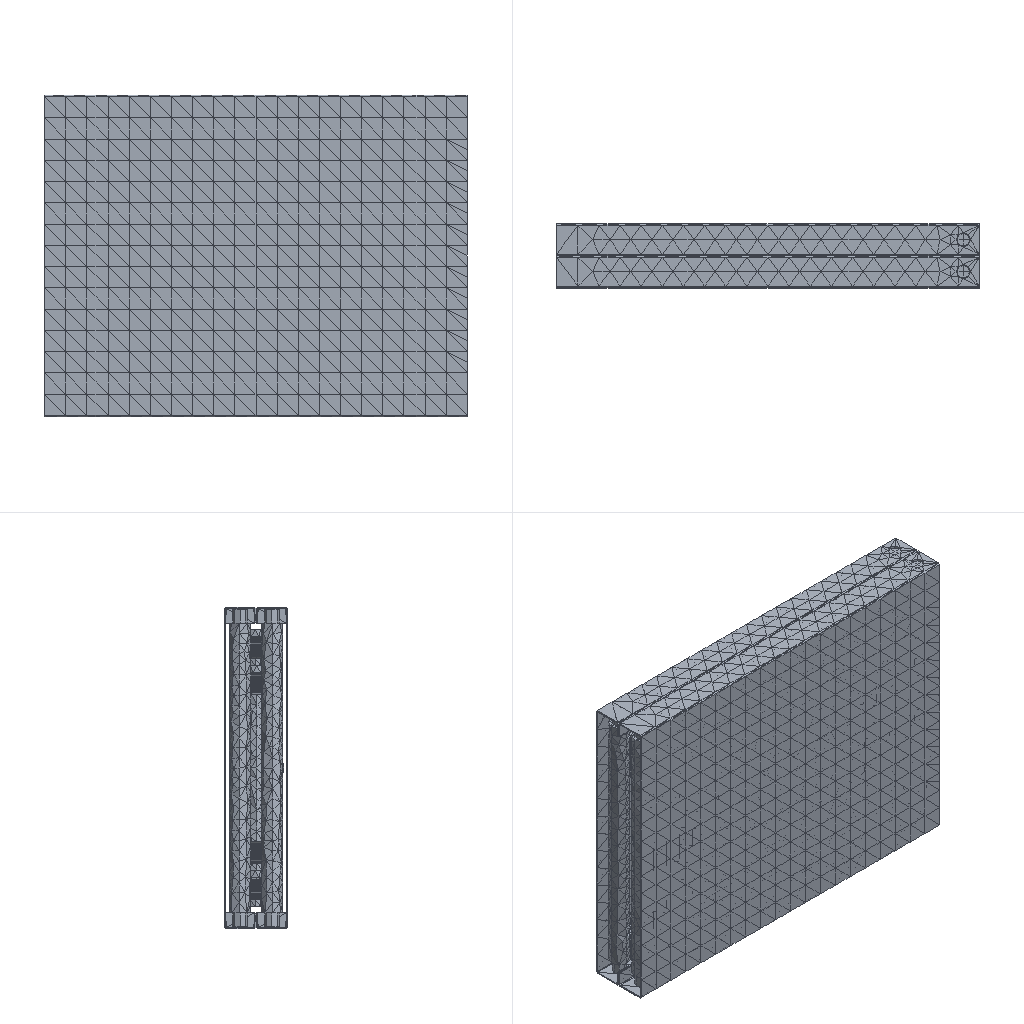Simulation study | abaqus
Set-up summary:
category,name,step,type,value,unit,region
solver,abaqus
solver,version,,,Abaqus/Explicit 2020
units,not stated in the deck,,not stated
analysis,deck,,transient,transient
load_step,Step-1,Step-1,transient
load_step,requested,,,1
mesh,nodes,,,15230
mesh,elements,,,42276
element_type,C3D4,,solid,41198
element_type,C3D8R,,solid,1078
load,load commands in deck,,count,3
bc,support commands in deck,,count,12
material,AI,,in results
check,setup vs results,,match,"per instance, exact: element labels, types and connectivity; labels of the nodes the elements use; coordinates not compared"
Abaqus input file, long lists of numbers shortened:
*Heading
** Job name: Job-1 Model name: Model-1
** Generated by: Abaqus/CAE 2020
*Preprint, echo=NO, model=NO, history=NO, contact=NO
**
** PARTS
**
*Part, name=WORK-1
*Node
      1,   7.262,   37.636,        -192.
      2,  0.8978,          35.,        -192.
** (205 more lines like these left out)
*Element, type=C3D8R
 1,  11,  12,  18,  10,   2,   3,   9,   1
 2,  14,  15,  18,  12,   5,   6,   9,   3
** (86 more lines like these left out)
*Nset, nset=Set-2, generate
   1,  207,    1
*Elset, elset=Set-2, generate
  1,  88,   1
** Section: Section-1
*Solid Section, elset=Set-2, material=AI
,
*End Part
**
*Part, name=WORK-2
*Node
      1,   49.212,   40.328,         -40.
      2,   47.261,   37.408,         -40.
** (872 more lines like these left out)
*Element, type=C3D8R
  1,  69,  42,  43,  56,  31,   4,   5,  18
  2,  43,  44,  70,  56,   5,   6,  32,  18
** (636 more lines like these left out)
*Nset, nset=Set-2, generate
   1,  874,    1
*Elset, elset=Set-2, generate
   1,  638,    1
** Section: Section-1
*Solid Section, elset=Set-2, material=AI
,
*End Part
**
*Part, name=WORK-3
*Node
      1,   221.697,    26.355,         13.5
      2,   221.697,    26.355,        -13.5
** (710 more lines like these left out)
*Element, type=C3D4
   1, 627, 628, 121, 610
   2, 627, 629, 630, 631
** (2272 more lines like these left out)
*Nset, nset=Set-4, generate
   1,  712,    1
*Elset, elset=Set-4, generate
    1,  2274,     1
** Section: Section-1
*Solid Section, elset=Set-4, material=AI
,
*End Part
**
*Part, name=WORK-4
*Node
      1,   220.068,   26.512,        -12.5
      2,   221.266,   38.955,           0.
** (209 more lines like these left out)
*Element, type=C3D4
  1, 191,  70,  71,  78
  2,  45, 192,  38,  37
** (585 more lines like these left out)
*Nset, nset=Set-4, generate
   1,  211,    1
*Elset, elset=Set-4, generate
   1,  587,    1
** Section: Section-1
*Solid Section, elset=Set-4, material=AI
,
*End Part
**
*Part, name=WORK-5
*Node
      1,  -261.84,   59.636,      -220.25
      2,  -268.204,          57.,      -220.25
** (205 more lines like these left out)
*Element, type=C3D8R
 1,  10,  11,  18,  13,   1,   2,   9,   4
 2,  17,  13,  18,  16,   8,   4,   9,   7
** (86 more lines like these left out)
*Nset, nset=Set-2, generate
   1,  207,    1
*Elset, elset=Set-2, generate
  1,  88,   1
** Section: Section-1
*Solid Section, elset=Set-2, material=AI
,
*End Part
**
*Part, name=WORK-6
*Node
      1,   276.364,   59.636,      -220.25
      2,         270.,          57.,      -220.25
** (205 more lines like these left out)
*Element, type=C3D8R
 1,  10,  11,  18,  13,   1,   2,   9,   4
 2,  12,  14,  18,  11,   3,   5,   9,   2
** (86 more lines like these left out)
*Nset, nset=Set-1, generate
   1,  207,    1
*Elset, elset=Set-1, generate
  1,  88,   1
** Section: Section-1
*Solid Section, elset=Set-1, material=AI
,
*End Part
**
*Part, name=WORK-7
*Node
      1,   276.364,   15.636,      -220.25
      2,         270.,          13.,      -220.25
** (205 more lines like these left out)
*Element, type=C3D8R
 1,  18,  11,  12,  14,   9,   2,   3,   5
 2,  10,  11,  18,  13,   1,   2,   9,   4
** (86 more lines like these left out)
*Nset, nset=Set-1, generate
   1,  207,    1
*Elset, elset=Set-1, generate
  1,  88,   1
** Section: Section-1
*Solid Section, elset=Set-1, material=AI
,
*End Part
**
*Part, name=WORK-8
*Node
      1,  -261.84,   15.636,      -220.25
      2,  -268.204,          13.,      -220.25
** (205 more lines like these left out)
*Element, type=C3D8R
 1,  18,  11,  12,  14,   9,   2,   3,   5
 2,  10,  11,  18,  13,   1,   2,   9,   4
** (86 more lines like these left out)
*Nset, nset=Set-1, generate
   1,  207,    1
*Elset, elset=Set-1, generate
  1,  88,   1
** Section: Section-1
*Solid Section, elset=Set-1, material=AI
,
*End Part
**
*Part, name=WORK-11
*Node
      1,         242.,          86.,      -200.25
      2,         242.,          86.,      -219.25
** (1151 more lines like these left out)
*Element, type=C3D4
   1, 1136,   63,   62,  243
   2,    7,   58,   10,   26
** (3214 more lines like these left out)
*Nset, nset=Set-1, generate
    1,  1153,     1
*Elset, elset=Set-1, generate
    1,  3216,     1
** Section: Section-1
*Solid Section, elset=Set-1, material=AI
,
*End Part
**
*Part, name=WORK-12
*Node
      1,  0.08297,   53.967,         142.
      2,  -9.069,   43.185,         142.
** (5124 more lines like these left out)
*Element, type=C3D4
    1, 4402, 1843, 4209, 1844
    2, 1441, 1803, 4209, 1804
** (16189 more lines like these left out)
*Nset, nset=Set-1, generate
    1,  5126,     1
*Elset, elset=Set-1, generate
     1,  16191,      1
** Section: Section-1
*Solid Section, elset=Set-1, material=AI
,
*End Part
**
*Part, name=WORK-15
*Node
      1,  -278.171,   66.815,       200.25
      2,  -258.238,   65.185,       200.25
** (4965 more lines like these left out)
*Element, type=C3D4
    1, 3918, 4688, 4421, 3917
    2, 4689, 3577, 4690, 4348
** (15720 more lines like these left out)
*Nset, nset=Set-1, generate
    1,  4967,     1
*Elset, elset=Set-1, generate
     1,  15722,      1
** Section: Section-1
*Solid Section, elset=Set-1, material=AI
,
*End Part
**
*Part, name=WORK-16
*Node
      1,         242.,           2.,       200.25
      2,         242.,           2.,       219.25
** (1150 more lines like these left out)
*Element, type=C3D4
   1,  388, 1136,   26,  407
   2, 1013,  790,  800,  999
** (3206 more lines like these left out)
*Nset, nset=Set-6, generate
    1,  1152,     1
*Elset, elset=Set-6, generate
    1,  3208,     1
** Section: Section-1
*Solid Section, elset=Set-6, material=AI
,
*End Part
**
**
** ASSEMBLY
**
*Assembly, name=Assembly
**
*Instance, name=WORK-1-1, part=WORK-1
*End Instance
**
*Instance, name=WORK-2-1, part=WORK-2
*End Instance
**
*Instance, name=WORK-3-1, part=WORK-3
*End Instance
**
*Instance, name=WORK-4-1, part=WORK-4
*End Instance
**
*Instance, name=WORK-5-1, part=WORK-5
*End Instance
**
*Instance, name=WORK-6-1, part=WORK-6
*End Instance
**
*Instance, name=WORK-7-1, part=WORK-7
*End Instance
**
*Instance, name=WORK-8-1, part=WORK-8
*End Instance
**
*Instance, name=WORK-11-1, part=WORK-11
*End Instance
**
*Instance, name=WORK-12-1, part=WORK-12
*End Instance
**
*Instance, name=WORK-15-1, part=WORK-15
*End Instance
**
*Instance, name=WORK-16-1, part=WORK-16
*End Instance
**
*Node
      1,           0.,         100.,           0.
*Nset, nset=Set-1, instance=WORK-16-1
   15,   16,   46,   47,   77,   78,   79,   80,   81,   82,   83,   84,   85,   86,   87,   88
   89,   90,  389,  390,  391,  392,  393,  394,  395,  396,  397,  398,  399,  400,  401,  402
** (20 more lines like these left out)
*Elset, elset=Set-1, instance=WORK-16-1
   19,   34,   38,   48,   50,  234,  236,  244,  245,  247,  248,  250,  252,  253,  254,  256
  260,  265,  266,  270,  272,  273,  274,  278,  279,  284,  290,  299,  308,  309,  313,  315
** (37 more lines like these left out)
*Nset, nset=Set-2, instance=WORK-11-1
   15,   16,   46,   47,   77,   78,   79,   80,   81,   82,   83,   84,   85,   86,   87,   88
   89,   90,  389,  390,  391,  392,  393,  394,  395,  396,  397,  398,  399,  400,  401,  402
** (20 more lines like these left out)
*Elset, elset=Set-2, instance=WORK-11-1
    7,    8,   60,   64,   67,   82,   94,  146,  261,  263,  266,  267,  276,  278,  279,  283
  284,  285,  287,  292,  297,  298,  302,  304,  310,  314,  315,  320,  322,  333,  336,  339
** (37 more lines like these left out)
*Nset, nset=Set-4
 1,
*Nset, nset=Set-5, instance=WORK-7-1
   1,   2,   3,   4,   5,   6,   7,   8,   9, 199, 200, 201, 202, 203, 204, 205
 206, 207
*Nset, nset=Set-5, instance=WORK-8-1
   1,   2,   3,   4,   5,   6,   7,   8,   9, 199, 200, 201, 202, 203, 204, 205
 206, 207
*Elset, elset=Set-5, instance=WORK-7-1
  1,  2,  3,  4, 85, 86, 87, 88
*Elset, elset=Set-5, instance=WORK-8-1
  1,  2,  3,  4, 85, 86, 87, 88
*Nset, nset=Set-6
 1,
*Nset, nset=m_Set-3
 1,
*Elset, elset=_m_Surf-1_S2, internal, instance=WORK-5-1, generate
 1,  4,  1
*Surface, type=ELEMENT, name=m_Surf-1
_m_Surf-1_S2, S2
*Elset, elset=_m_Surf-3_S1, internal, instance=WORK-5-1, generate
 85,  88,   1
*Surface, type=ELEMENT, name=m_Surf-3
_m_Surf-3_S1, S1
*Elset, elset=_m_Surf-5_S1, internal, instance=WORK-8-1, generate
 85,  88,   1
*Surface, type=ELEMENT, name=m_Surf-5
_m_Surf-5_S1, S1
*Elset, elset=_m_Surf-7_S2, internal, instance=WORK-8-1, generate
 1,  4,  1
*Surface, type=ELEMENT, name=m_Surf-7
_m_Surf-7_S2, S2
*Elset, elset=_m_Surf-9_S2, internal, instance=WORK-1-1, generate
 1,  4,  1
*Surface, type=ELEMENT, name=m_Surf-9
_m_Surf-9_S2, S2
*Elset, elset=_m_Surf-11_S1, internal, instance=WORK-1-1, generate
 85,  88,   1
*Surface, type=ELEMENT, name=m_Surf-11
_m_Surf-11_S1, S1
*Elset, elset=_m_Surf-13_S1, internal, instance=WORK-2-1, generate
 610,  638,    1
*Surface, type=ELEMENT, name=m_Surf-13
_m_Surf-13_S1, S1
*Elset, elset=_m_Surf-15_S2, internal, instance=WORK-2-1, generate
  1,  29,   1
*Surface, type=ELEMENT, name=m_Surf-15
_m_Surf-15_S2, S2
*Elset, elset=_m_Surf-17_S2, internal, instance=WORK-7-1, generate
 1,  4,  1
*Surface, type=ELEMENT, name=m_Surf-17
_m_Surf-17_S2, S2
*Elset, elset=_m_Surf-19_S1, internal, instance=WORK-7-1, generate
 85,  88,   1
*Surface, type=ELEMENT, name=m_Surf-19
_m_Surf-19_S1, S1
*Elset, elset=_m_Surf-22_S3, internal, instance=WORK-11-1
 1265, 1636, 1824, 1874, 1936, 1947, 1950, 1954, 1958, 1963, 1969, 1971, 1973, 1976, 1979, 1980
 1982, 1983, 1986, 1988, 1991, 1998, 2003, 2005, 2006, 2008, 2025, 2251, 2301, 2337, 2634, 3199
*Elset, elset=_m_Surf-22_S1, internal, instance=WORK-11-1
 1934,
*Elset, elset=_m_Surf-22_S4, internal, instance=WORK-11-1
 1941, 2218, 2557
*Surface, type=ELEMENT, name=m_Surf-22
_m_Surf-22_S3, S3
_m_Surf-22_S1, S1
_m_Surf-22_S4, S4
*Elset, elset=_s_Surf-9_S3, internal, instance=WORK-15-1
   19,   20, 4468, 8664, 8738, 9003
*Elset, elset=_s_Surf-9_S4, internal, instance=WORK-15-1
   917,  8114,  8551,  8679,  8687,  8734,  9651, 12450
*Elset, elset=_s_Surf-9_S2, internal, instance=WORK-15-1
  7329,  8970, 11381, 14219
*Elset, elset=_s_Surf-9_S1, internal, instance=WORK-15-1
 9655,
*Surface, type=ELEMENT, name=s_Surf-9
_s_Surf-9_S3, S3
_s_Surf-9_S4, S4
_s_Surf-9_S2, S2
_s_Surf-9_S1, S1
*Elset, elset=_s_Surf-11_S3, internal, instance=WORK-15-1
   204,  1697,  6734,  7453,  8763,  8825,  8840,  9844,  9986,  9988,  9997,  9998, 10074, 10289
*Elset, elset=_s_Surf-11_S4, internal, instance=WORK-15-1
   654,  1522,  9991, 10290
*Elset, elset=_s_Surf-11_S1, internal, instance=WORK-15-1
 12418,
*Surface, type=ELEMENT, name=s_Surf-11
_s_Surf-11_S3, S3
_s_Surf-11_S4, S4
_s_Surf-11_S1, S1
*Elset, elset=_s_Surf-13_S3, internal, instance=WORK-12-1
    39,   233,   457,  1169,  1170,  9256,  9276,  9284,  9342,  9351,  9464,  9510,  9515,  9607,  9940, 11445
 11625,
*Elset, elset=_s_Surf-13_S2, internal, instance=WORK-12-1
 440,
*Elset, elset=_s_Surf-13_S1, internal, instance=WORK-12-1
  442, 9272
*Elset, elset=_s_Surf-13_S4, internal, instance=WORK-12-1
  1168,  9617,  9901, 11439
*Surface, type=ELEMENT, name=s_Surf-13
_s_Surf-13_S3, S3
_s_Surf-13_S2, S2
_s_Surf-13_S4, S4
_s_Surf-13_S1, S1
*Elset, elset=_s_Surf-15_S4, internal, instance=WORK-12-1
    30,  7769,  7956, 12024, 15156
*Elset, elset=_s_Surf-15_S3, internal, instance=WORK-12-1
    77,   187,  1341,  3155,  5025,  5391,  6906,  6913,  7975, 10011, 12041, 15675, 15787, 15804, 15808, 15815
 15823,
*Elset, elset=_s_Surf-15_S2, internal, instance=WORK-12-1
 5422,
*Elset, elset=_s_Surf-15_S1, internal, instance=WORK-12-1
 15677,
*Surface, type=ELEMENT, name=s_Surf-15
_s_Surf-15_S4, S4
_s_Surf-15_S3, S3
_s_Surf-15_S2, S2
_s_Surf-15_S1, S1
*Elset, elset=_s_Surf-17_S4, internal, instance=WORK-16-1
   36,  121,  125,  128,  145,  146,  147,  148,  150,  167,  170,  171,  173,  179,  187,  208
  209,  217,  221,  224,  846, 1879, 1990, 2024, 2135, 2240, 2241, 2579, 2637, 2670, 2681, 2712
** (1 more lines like these left out)
*Elset, elset=_s_Surf-17_S3, internal, instance=WORK-16-1
   51,   55,   76,  158,  169,  175,  211,  769, 2086, 2108, 2157, 2160, 2552
*Elset, elset=_s_Surf-17_S1, internal, instance=WORK-16-1
   68,  116,  186,  188,  191,  214,  996, 1421, 1827, 2286, 2642, 2690, 2727, 2981, 2986, 2987
 2997, 3037
*Elset, elset=_s_Surf-17_S2, internal, instance=WORK-16-1
   89,  124,  140,  168,  184,  192,  199,  218,  222,  267,  351,  480, 1050, 1137, 2080, 2536
 2555, 2583, 2892, 2896, 2897, 2954, 2959
*Surface, type=ELEMENT, name=s_Surf-17
_s_Surf-17_S4, S4
_s_Surf-17_S3, S3
_s_Surf-17_S2, S2
_s_Surf-17_S1, S1
*Elset, elset=_s_Surf-19_S3, internal, instance=WORK-16-1
   21,   74,   75,  924, 1760, 1906, 1979, 2199
*Elset, elset=_s_Surf-19_S2, internal, instance=WORK-16-1
  511, 1047, 1707, 1711, 1715, 1719, 1723, 1728, 1751, 1828, 1851, 1893, 1897, 1957, 1959, 1971
 1974, 2015, 2151, 2190, 2360, 2384
*Elset, elset=_s_Surf-19_S4, internal, instance=WORK-16-1
  607, 1714, 1741, 1782, 1792, 1794, 1802, 1818, 1835, 1853, 1868, 1875, 1907, 1910, 1922, 1926
 1949, 1953, 1996, 2019, 2025, 2105, 2269, 2296, 2301, 2303, 2308, 2317, 2321, 2325, 3136
*Elset, elset=_s_Surf-19_S1, internal, instance=WORK-16-1
 1708, 1709, 1718, 1722, 1732, 1735, 1742, 1744, 1750, 1769, 1780, 1781, 1785, 1805, 1809, 1813
 1816, 1819, 1837, 1925, 1928, 1938, 1972, 1993, 2014, 2282, 2351, 2387, 2851
*Surface, type=ELEMENT, name=s_Surf-19
_s_Surf-19_S3, S3
_s_Surf-19_S2, S2
_s_Surf-19_S4, S4
_s_Surf-19_S1, S1
*Elset, elset=_s_Surf-21_S3, internal, instance=WORK-11-1
    7,    8,  298,  302,  310,  320,  322,  339,  409,  512,  548,  563,  621,  648,  670,  699
  740,  760,  786,  845,  847,  850,  854,  896,  924,  985, 1007, 1041, 1070, 1074, 1110, 1133
** (3 more lines like these left out)
*Elset, elset=_s_Surf-21_S2, internal, instance=WORK-11-1
   60,   67,   82,   94,  146,  261,  263,  278,  285,  287,  292,  297,  314,  341,  349,  350
  357,  362,  365,  371,  372,  374,  381,  383,  388,  399,  402,  419,  423,  427,  433,  439
** (12 more lines like these left out)
*Elset, elset=_s_Surf-21_S4, internal, instance=WORK-11-1
   64,  266,  283,  304,  315,  333,  354,  360,  369,  375,  380,  384,  385,  407,  443,  477
  487,  493,  518,  524,  532,  547,  564,  586,  590,  627,  654,  669,  678,  679,  681,  707
** (7 more lines like these left out)
*Elset, elset=_s_Surf-21_S1, internal, instance=WORK-11-1
  267,  276,  279,  284,  336,  344,  364,  391,  397,  404,  429,  448,  459,  467,  474,  508
  509,  515,  520,  535,  541,  574,  583,  594,  615,  622,  624,  625,  634,  693,  708,  709
** (9 more lines like these left out)
*Surface, type=ELEMENT, name=s_Surf-21
_s_Surf-21_S3, S3
_s_Surf-21_S2, S2
_s_Surf-21_S4, S4
_s_Surf-21_S1, S1
*Elset, elset=_s_Surf-22_S1, internal, instance=WORK-5-1, generate
 85,  88,   1
*Elset, elset=_s_Surf-22_S1, internal, instance=WORK-6-1, generate
 85,  88,   1
*Elset, elset=_s_Surf-22_S2, internal, instance=WORK-5-1, generate
 1,  4,  1
*Elset, elset=_s_Surf-22_S2, internal, instance=WORK-6-1, generate
 1,  4,  1
*Surface, type=ELEMENT, name=s_Surf-22
_s_Surf-22_S1, S1
_s_Surf-22_S2, S2
** Constraint: Constraint-1
*Tie, name=Constraint-1, adjust=yes
s_Surf-22, m_Surf-22
** Constraint: Constraint-5
*Tie, name=Constraint-5, adjust=yes
s_Surf-9, m_Surf-9
** Constraint: Constraint-6
*Tie, name=Constraint-6, adjust=yes
s_Surf-11, m_Surf-11
** Constraint: Constraint-7
*Tie, name=Constraint-7, adjust=yes
s_Surf-13, m_Surf-13
** Constraint: Constraint-8
*Tie, name=Constraint-8, adjust=yes
s_Surf-15, m_Surf-15
** Constraint: v
*Coupling, constraint name=v, ref node=m_Set-3, surface=s_Surf-21
*Kinematic
*End Assembly
**
** MATERIALS
**
*Material, name=AI
*Density
 2.8e-09,
*Elastic
70000., 0.33
**
** INTERACTION PROPERTIES
**
*Surface Interaction, name=IntProp-1
*Friction
 0.3,
*Surface Behavior, pressure-overclosure=HARD
** ----------------------------------------------------------------
**
** STEP: Step-1
**
*Step, name=Step-1, nlgeom=YES
*Dynamic, Explicit
, 4.
*Bulk Viscosity
0.06, 1.2
** Mass Scaling: Semi-Automatic
**               Whole Model
*Fixed Mass Scaling, dt=1e-05, type=below min
**
** BOUNDARY CONDITIONS
**
** Name: BC-1 Type: 对称/反对称/完全固定
*Boundary
Set-1, ENCASTRE
** Name: BC-3 Type: 位移/转角
*Boundary
Set-5, 2, 2
Set-5, 3, 3
Set-5, 4, 4
Set-5, 5, 5
Set-5, 6, 6
** Name: v Type: velocity/angular velocity
*Boundary, type=VELOCITY
Set-4, 1, 1
Set-4, 2, 2, 50.
Set-4, 3, 3
Set-4, 4, 4
Set-4, 5, 5
Set-4, 6, 6
**
** LOADS
**
** Name: Load-1   Type: Gravity
*Dload
, GRAV, 9800., 0., -1., 0.
** Name: Load-2   Type: Concentrated force
*Cload
Set-6, 2, -1760.
**
** INTERACTIONS
**
** Interaction: Int-1
*Contact, op=NEW
*Contact Inclusions, ALL EXTERIOR
*Contact Property Assignment
 ,  , IntProp-1
**
** OUTPUT REQUESTS
**
*Restart, write, number interval=1, time marks=NO
**
** FIELD OUTPUT: F-Output-1
**
*Output, field, number interval=200
*Node Output
A, RF, U, V
*Element Output, directions=YES
E, LE, MISES, PE, PEEQ, PEEQVAVG, PEVAVG, S, SVAVG
*Contact Output
CSTRESS,
**
** HISTORY OUTPUT: H-Output-1
**
*Output, history, variable=PRESELECT
*End Step
Results summary:
result,step,Step-1,partial,increments=309541 time=3.122/4.0
result,analysis,,,transient
result,last_loadstep,,,1
result,primary field,,,U
result,reaction total,,FX,7613.599,model units
result,reaction total,,FY,2543.561,model units
result,reaction total,,FZ,-1527.832,model units